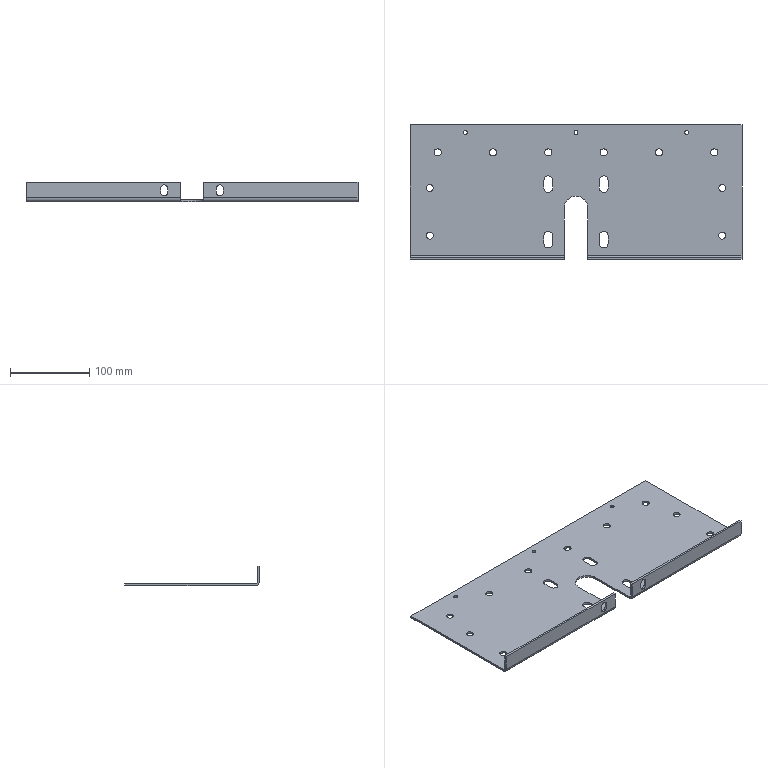Part | STEP file | cc-roller-motor section | 1 solid | 55 faces | box 418.8 x 170 x 25 mm | volume 188211 mm3 | plane 25 | cylinder 16 | spline 14 | commonest cylinder face diameters 11 x8 9 x4 5 x2 10 x2